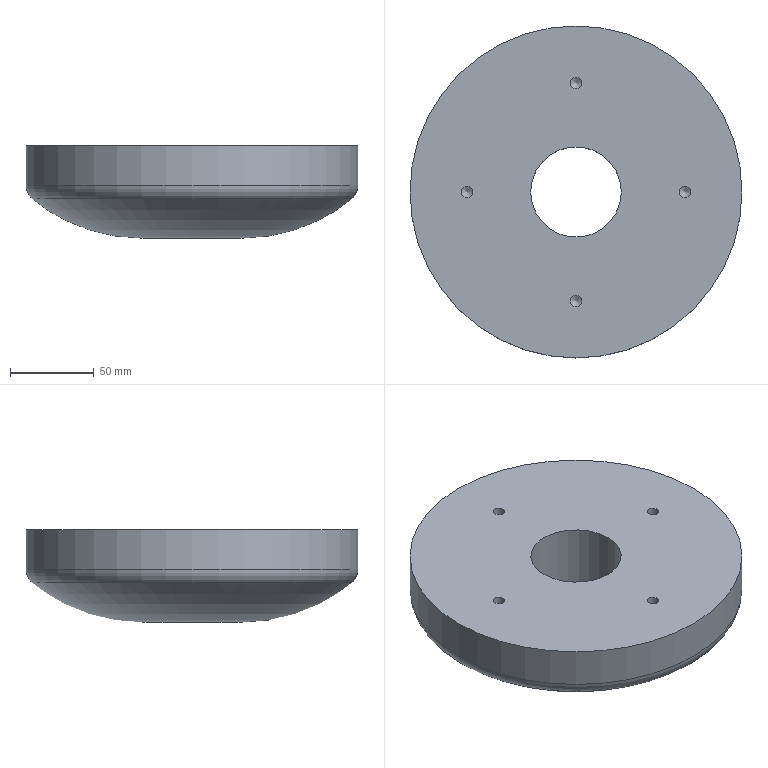Part | STEP file | JBJ-P-1000-04 | 1 solid | 14 faces | box 198 x 198 x 55 mm | volume 1265765 mm3 | cylinder 6 | cone 4 | plane 2 | torus 2 | commonest cylinder face diameters 6.8 x4 54 x1 198 x1
STEP:
#1=CARTESIAN_POINT('',(27.,0.,0.));
#2=VERTEX_POINT('',#1);
#3=CARTESIAN_POINT('',(0.,0.,0.));
#4=DIRECTION('',(0.,0.,1.));
#5=DIRECTION('',(1.,0.,0.));
#6=AXIS2_PLACEMENT_3D('',#3,#4,#5);
#7=CIRCLE('',#6,27.);
#8=EDGE_CURVE('',#2,#2,#7,.T.);
#9=ORIENTED_EDGE('',*,*,#8,.F.);
#10=EDGE_LOOP('',(#9));
#11=FACE_BOUND('',#10,.T.);
#12=CARTESIAN_POINT('',(3.4,65.,0.));
#13=VERTEX_POINT('',#12);
#14=CARTESIAN_POINT('',(0.,65.,0.));
#15=DIRECTION('',(0.,0.,1.));
#16=DIRECTION('',(1.,0.,0.));
#17=AXIS2_PLACEMENT_3D('',#14,#15,#16);
#18=CIRCLE('',#17,3.4);
#19=EDGE_CURVE('',#13,#13,#18,.T.);
#20=ORIENTED_EDGE('',*,*,#19,.F.);
#21=EDGE_LOOP('',(#20));
#22=FACE_BOUND('',#21,.T.);
#23=CARTESIAN_POINT('',(68.4,0.,0.));
#24=VERTEX_POINT('',#23);
#25=CARTESIAN_POINT('',(65.,0.,0.));
#26=DIRECTION('',(0.,0.,1.));
#27=DIRECTION('',(1.,0.,0.));
#28=AXIS2_PLACEMENT_3D('',#25,#26,#27);
#29=CIRCLE('',#28,3.4);
#30=EDGE_CURVE('',#24,#24,#29,.T.);
#31=ORIENTED_EDGE('',*,*,#30,.F.);
#32=EDGE_LOOP('',(#31));
#33=FACE_BOUND('',#32,.T.);
#34=CARTESIAN_POINT('',(3.4,-65.,0.));
#35=VERTEX_POINT('',#34);
#36=CARTESIAN_POINT('',(0.,-65.,0.));
#37=DIRECTION('',(0.,0.,1.));
#38=DIRECTION('',(1.,0.,0.));
#39=AXIS2_PLACEMENT_3D('',#36,#37,#38);
#40=CIRCLE('',#39,3.4);
#41=EDGE_CURVE('',#35,#35,#40,.T.);
#42=ORIENTED_EDGE('',*,*,#41,.F.);
#43=EDGE_LOOP('',(#42));
#44=FACE_BOUND('',#43,.T.);
#45=CARTESIAN_POINT('',(-61.6,0.,0.));
#46=VERTEX_POINT('',#45);
#47=CARTESIAN_POINT('',(-65.,0.,0.));
#48=DIRECTION('',(0.,0.,1.));
#49=DIRECTION('',(1.,0.,0.));
#50=AXIS2_PLACEMENT_3D('',#47,#48,#49);
#51=CIRCLE('',#50,3.4);
#52=EDGE_CURVE('',#46,#46,#51,.T.);
#53=ORIENTED_EDGE('',*,*,#52,.F.);
#54=EDGE_LOOP('',(#53));
#55=FACE_BOUND('',#54,.T.);
#56=CARTESIAN_POINT('',(99.,0.,0.));
#57=VERTEX_POINT('',#56);
#58=CARTESIAN_POINT('',(0.,0.,0.));
#59=DIRECTION('',(0.,0.,1.));
#60=DIRECTION('',(1.,0.,0.));
#61=AXIS2_PLACEMENT_3D('',#58,#59,#60);
#62=CIRCLE('',#61,99.);
#63=EDGE_CURVE('',#57,#57,#62,.T.);
#64=ORIENTED_EDGE('',*,*,#63,.T.);
#65=EDGE_LOOP('',(#64));
#66=FACE_OUTER_BOUND('',#65,.T.);
#67=CARTESIAN_POINT('',(-99.,0.,0.));
#68=DIRECTION('',(0.,0.,-1.));
#69=DIRECTION('',(-1.,0.,0.));
#70=AXIS2_PLACEMENT_3D('',#67,#68,#69);
#71=PLANE('',#70);
#72=ADVANCED_FACE('',(#11,#22,#33,#44,#55,#66),#71,.F.);
#73=CARTESIAN_POINT('',(27.,0.,-55.));
#74=VERTEX_POINT('',#73);
#75=CARTESIAN_POINT('',(0.,0.,-55.));
#76=DIRECTION('',(0.,0.,1.));
#77=DIRECTION('',(1.,0.,0.));
#78=AXIS2_PLACEMENT_3D('',#75,#76,#77);
#79=CIRCLE('',#78,27.);
#80=EDGE_CURVE('',#74,#74,#79,.T.);
#81=ORIENTED_EDGE('',*,*,#80,.T.);
#82=EDGE_LOOP('',(#81));
#83=FACE_BOUND('',#82,.T.);
#84=CARTESIAN_POINT('',(29.998,0.,-55.));
#85=VERTEX_POINT('',#84);
#86=CARTESIAN_POINT('',(0.,0.,-55.));
#87=DIRECTION('',(0.,0.,1.));
#88=DIRECTION('',(1.,0.,0.));
#89=AXIS2_PLACEMENT_3D('',#86,#87,#88);
#90=CIRCLE('',#89,29.998);
#91=EDGE_CURVE('',#85,#85,#90,.T.);
#92=ORIENTED_EDGE('',*,*,#91,.F.);
#93=EDGE_LOOP('',(#92));
#94=FACE_OUTER_BOUND('',#93,.T.);
#95=CARTESIAN_POINT('',(-29.998,0.,-55.));
#96=DIRECTION('',(0.,0.,1.));
#97=DIRECTION('',(1.,0.,0.));
#98=AXIS2_PLACEMENT_3D('',#95,#96,#97);
#99=PLANE('',#98);
#100=ADVANCED_FACE('',(#83,#94),#99,.F.);
#101=CARTESIAN_POINT('',(95.358,0.,-31.547));
#102=VERTEX_POINT('',#101);
#103=CARTESIAN_POINT('',(0.,0.,-31.547));
#104=DIRECTION('',(0.,0.,1.));
#105=DIRECTION('',(1.,0.,0.));
#106=AXIS2_PLACEMENT_3D('',#103,#104,#105);
#107=CIRCLE('',#106,95.358);
#108=EDGE_CURVE('',#102,#102,#107,.T.);
#109=ORIENTED_EDGE('',*,*,#108,.F.);
#110=EDGE_LOOP('',(#109));
#111=FACE_OUTER_BOUND('',#110,.T.);
#112=ORIENTED_EDGE('',*,*,#91,.T.);
#113=EDGE_LOOP('',(#112));
#114=FACE_OUTER_BOUND('',#113,.T.);
#115=CARTESIAN_POINT('',(0.,0.,47.8));
#116=DIRECTION('',(0.,0.,1.));
#117=DIRECTION('',(1.,0.,0.));
#118=AXIS2_PLACEMENT_3D('',#115,#116,#117);
#119=TOROIDAL_SURFACE('',#118,29.998,102.8);
#120=ADVANCED_FACE('',(#111,#114),#119,.T.);
#121=CARTESIAN_POINT('',(99.,0.,-23.828));
#122=VERTEX_POINT('',#121);
#123=CARTESIAN_POINT('',(0.,0.,-23.828));
#124=DIRECTION('',(0.,0.,1.));
#125=DIRECTION('',(1.,0.,0.));
#126=AXIS2_PLACEMENT_3D('',#123,#124,#125);
#127=CIRCLE('',#126,99.);
#128=EDGE_CURVE('',#122,#122,#127,.T.);
#129=ORIENTED_EDGE('',*,*,#128,.F.);
#130=EDGE_LOOP('',(#129));
#131=FACE_OUTER_BOUND('',#130,.T.);
#132=ORIENTED_EDGE('',*,*,#108,.T.);
#133=EDGE_LOOP('',(#132));
#134=FACE_OUTER_BOUND('',#133,.T.);
#135=CARTESIAN_POINT('',(0.,0.,-23.828));
#136=DIRECTION('',(0.,0.,1.));
#137=DIRECTION('',(1.,0.,0.));
#138=AXIS2_PLACEMENT_3D('',#135,#136,#137);
#139=TOROIDAL_SURFACE('',#138,89.,10.);
#140=ADVANCED_FACE('',(#131,#134),#139,.T.);
#141=ORIENTED_EDGE('',*,*,#63,.F.);
#142=EDGE_LOOP('',(#141));
#143=FACE_OUTER_BOUND('',#142,.T.);
#144=ORIENTED_EDGE('',*,*,#128,.T.);
#145=EDGE_LOOP('',(#144));
#146=FACE_OUTER_BOUND('',#145,.T.);
#147=CARTESIAN_POINT('',(0.,0.,0.));
#148=DIRECTION('',(0.,0.,1.));
#149=DIRECTION('',(1.,0.,0.));
#150=AXIS2_PLACEMENT_3D('',#147,#148,#149);
#151=CYLINDRICAL_SURFACE('',#150,99.);
#152=ADVANCED_FACE('',(#143,#146),#151,.T.);
#153=CARTESIAN_POINT('',(-61.6,0.,-15.));
#154=VERTEX_POINT('',#153);
#155=CARTESIAN_POINT('',(-65.,0.,-15.));
#156=DIRECTION('',(0.,0.,1.));
#157=DIRECTION('',(1.,0.,0.));
#158=AXIS2_PLACEMENT_3D('',#155,#156,#157);
#159=CIRCLE('',#158,3.4);
#160=EDGE_CURVE('',#154,#154,#159,.T.);
#161=ORIENTED_EDGE('',*,*,#160,.T.);
#162=EDGE_LOOP('',(#161));
#163=FACE_OUTER_BOUND('',#162,.T.);
#164=CARTESIAN_POINT('',(-65.,0.,-15.));
#165=DIRECTION('',(0.,0.,1.));
#166=DIRECTION('',(1.,0.,0.));
#167=AXIS2_PLACEMENT_3D('',#164,#165,#166);
#168=CONICAL_SURFACE('',#167,3.4,1.03);
#169=ADVANCED_FACE('',(#163),#168,.F.);
#170=ORIENTED_EDGE('',*,*,#160,.F.);
#171=EDGE_LOOP('',(#170));
#172=FACE_OUTER_BOUND('',#171,.T.);
#173=ORIENTED_EDGE('',*,*,#52,.T.);
#174=EDGE_LOOP('',(#173));
#175=FACE_OUTER_BOUND('',#174,.T.);
#176=CARTESIAN_POINT('',(-65.,0.,0.));
#177=DIRECTION('',(0.,0.,1.));
#178=DIRECTION('',(1.,0.,0.));
#179=AXIS2_PLACEMENT_3D('',#176,#177,#178);
#180=CYLINDRICAL_SURFACE('',#179,3.4);
#181=ADVANCED_FACE('',(#172,#175),#180,.F.);
#182=CARTESIAN_POINT('',(3.4,-65.,-15.));
#183=VERTEX_POINT('',#182);
#184=CARTESIAN_POINT('',(0.,-65.,-15.));
#185=DIRECTION('',(0.,0.,1.));
#186=DIRECTION('',(1.,0.,0.));
#187=AXIS2_PLACEMENT_3D('',#184,#185,#186);
#188=CIRCLE('',#187,3.4);
#189=EDGE_CURVE('',#183,#183,#188,.T.);
#190=ORIENTED_EDGE('',*,*,#189,.T.);
#191=EDGE_LOOP('',(#190));
#192=FACE_OUTER_BOUND('',#191,.T.);
#193=CARTESIAN_POINT('',(0.,-65.,-15.));
#194=DIRECTION('',(0.,0.,1.));
#195=DIRECTION('',(1.,0.,0.));
#196=AXIS2_PLACEMENT_3D('',#193,#194,#195);
#197=CONICAL_SURFACE('',#196,3.4,1.03);
#198=ADVANCED_FACE('',(#192),#197,.F.);
#199=ORIENTED_EDGE('',*,*,#189,.F.);
#200=EDGE_LOOP('',(#199));
#201=FACE_OUTER_BOUND('',#200,.T.);
#202=ORIENTED_EDGE('',*,*,#41,.T.);
#203=EDGE_LOOP('',(#202));
#204=FACE_OUTER_BOUND('',#203,.T.);
#205=CARTESIAN_POINT('',(0.,-65.,0.));
#206=DIRECTION('',(0.,0.,1.));
#207=DIRECTION('',(1.,0.,0.));
#208=AXIS2_PLACEMENT_3D('',#205,#206,#207);
#209=CYLINDRICAL_SURFACE('',#208,3.4);
#210=ADVANCED_FACE('',(#201,#204),#209,.F.);
#211=CARTESIAN_POINT('',(68.4,0.,-15.));
#212=VERTEX_POINT('',#211);
#213=CARTESIAN_POINT('',(65.,0.,-15.));
#214=DIRECTION('',(0.,0.,1.));
#215=DIRECTION('',(1.,0.,0.));
#216=AXIS2_PLACEMENT_3D('',#213,#214,#215);
#217=CIRCLE('',#216,3.4);
#218=EDGE_CURVE('',#212,#212,#217,.T.);
#219=ORIENTED_EDGE('',*,*,#218,.T.);
#220=EDGE_LOOP('',(#219));
#221=FACE_OUTER_BOUND('',#220,.T.);
#222=CARTESIAN_POINT('',(65.,0.,-15.));
#223=DIRECTION('',(0.,0.,1.));
#224=DIRECTION('',(1.,0.,0.));
#225=AXIS2_PLACEMENT_3D('',#222,#223,#224);
#226=CONICAL_SURFACE('',#225,3.4,1.03);
#227=ADVANCED_FACE('',(#221),#226,.F.);
#228=ORIENTED_EDGE('',*,*,#218,.F.);
#229=EDGE_LOOP('',(#228));
#230=FACE_OUTER_BOUND('',#229,.T.);
#231=ORIENTED_EDGE('',*,*,#30,.T.);
#232=EDGE_LOOP('',(#231));
#233=FACE_OUTER_BOUND('',#232,.T.);
#234=CARTESIAN_POINT('',(65.,0.,0.));
#235=DIRECTION('',(0.,0.,1.));
#236=DIRECTION('',(1.,0.,0.));
#237=AXIS2_PLACEMENT_3D('',#234,#235,#236);
#238=CYLINDRICAL_SURFACE('',#237,3.4);
#239=ADVANCED_FACE('',(#230,#233),#238,.F.);
#240=CARTESIAN_POINT('',(3.4,65.,-15.));
#241=VERTEX_POINT('',#240);
#242=CARTESIAN_POINT('',(0.,65.,-15.));
#243=DIRECTION('',(0.,0.,1.));
#244=DIRECTION('',(1.,0.,0.));
#245=AXIS2_PLACEMENT_3D('',#242,#243,#244);
#246=CIRCLE('',#245,3.4);
#247=EDGE_CURVE('',#241,#241,#246,.T.);
#248=ORIENTED_EDGE('',*,*,#247,.T.);
#249=EDGE_LOOP('',(#248));
#250=FACE_OUTER_BOUND('',#249,.T.);
#251=CARTESIAN_POINT('',(0.,65.,-15.));
#252=DIRECTION('',(0.,0.,1.));
#253=DIRECTION('',(1.,0.,0.));
#254=AXIS2_PLACEMENT_3D('',#251,#252,#253);
#255=CONICAL_SURFACE('',#254,3.4,1.03);
#256=ADVANCED_FACE('',(#250),#255,.F.);
#257=ORIENTED_EDGE('',*,*,#247,.F.);
#258=EDGE_LOOP('',(#257));
#259=FACE_OUTER_BOUND('',#258,.T.);
#260=ORIENTED_EDGE('',*,*,#19,.T.);
#261=EDGE_LOOP('',(#260));
#262=FACE_OUTER_BOUND('',#261,.T.);
#263=CARTESIAN_POINT('',(0.,65.,0.));
#264=DIRECTION('',(0.,0.,1.));
#265=DIRECTION('',(1.,0.,0.));
#266=AXIS2_PLACEMENT_3D('',#263,#264,#265);
#267=CYLINDRICAL_SURFACE('',#266,3.4);
#268=ADVANCED_FACE('',(#259,#262),#267,.F.);
#269=ORIENTED_EDGE('',*,*,#80,.F.);
#270=EDGE_LOOP('',(#269));
#271=FACE_OUTER_BOUND('',#270,.T.);
#272=ORIENTED_EDGE('',*,*,#8,.T.);
#273=EDGE_LOOP('',(#272));
#274=FACE_OUTER_BOUND('',#273,.T.);
#275=CARTESIAN_POINT('',(0.,0.,-55.));
#276=DIRECTION('',(0.,0.,1.));
#277=DIRECTION('',(1.,0.,0.));
#278=AXIS2_PLACEMENT_3D('',#275,#276,#277);
#279=CYLINDRICAL_SURFACE('',#278,27.);
#280=ADVANCED_FACE('',(#271,#274),#279,.F.);
#281=CLOSED_SHELL('',(#72,#100,#120,#140,#152,#169,#181,#198,#210,#227,#239,#256,#268,#280));
#282=MANIFOLD_SOLID_BREP('',#281);
#283=CARTESIAN_POINT('',(0.,0.,0.));
#284=DIRECTION('',(0.,0.,1.));
#285=DIRECTION('',(1.,0.,0.));
#286=AXIS2_PLACEMENT_3D('',#283,#284,#285);
#287=(LENGTH_UNIT()NAMED_UNIT(*)SI_UNIT(.MILLI.,.METRE.));
#288=UNCERTAINTY_MEASURE_WITH_UNIT(LENGTH_MEASURE(0.00001),#287,'','');
#289=(NAMED_UNIT(*)PLANE_ANGLE_UNIT()SI_UNIT($,.RADIAN.));
#290=(NAMED_UNIT(*)SI_UNIT($,.STERADIAN.)SOLID_ANGLE_UNIT());
#291=(GEOMETRIC_REPRESENTATION_CONTEXT(3)GLOBAL_UNCERTAINTY_ASSIGNED_CONTEXT((#288))GLOBAL_UNIT_ASSIGNED_CONTEXT((#287,#289,#290))REPRESENTATION_CONTEXT('',''));
#292=ADVANCED_BREP_SHAPE_REPRESENTATION('',(#282,#286),#291);